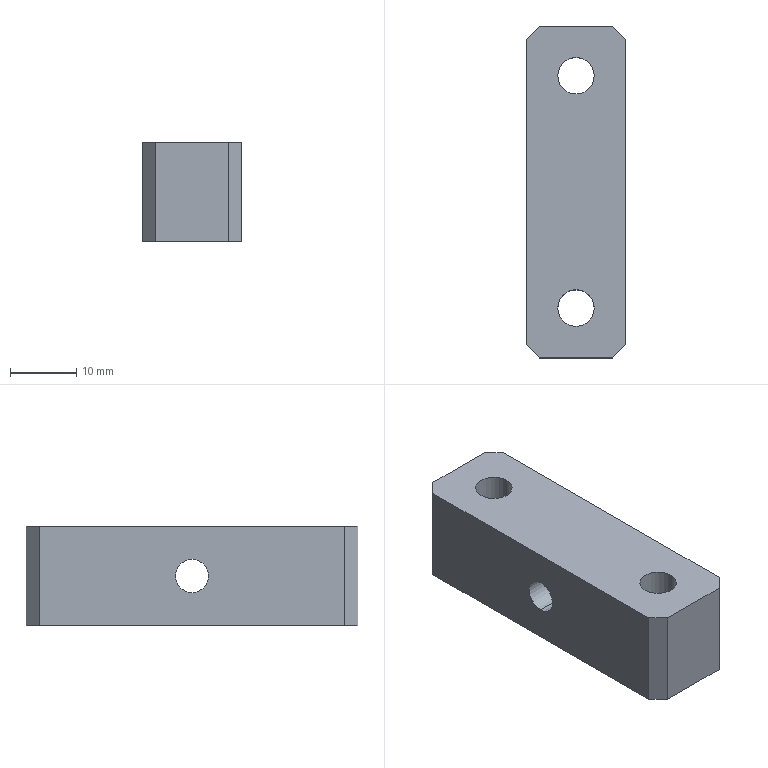Part | STEP file | MT-COMBO-119-S024 | 1 solid | 16 faces | box 15 x 50 x 15 mm | volume 10123 mm3 | plane 10 | cylinder 6 | commonest cylinder face diameters 5.5 x4 5 x2
STEP:
#1=CARTESIAN_POINT('',(0.,25.,5.));
#2=VERTEX_POINT('',#1);
#3=CARTESIAN_POINT('',(0.,25.,10.));
#4=VERTEX_POINT('',#3);
#5=CARTESIAN_POINT('',(0.,25.,7.5));
#6=DIRECTION('',(-1.,0.,0.));
#7=DIRECTION('',(0.,0.,1.));
#8=AXIS2_PLACEMENT_3D('',#5,#6,#7);
#9=CIRCLE('',#8,2.5);
#10=EDGE_CURVE('',#2,#4,#9,.T.);
#11=ORIENTED_EDGE('',*,*,#10,.F.);
#12=CARTESIAN_POINT('',(-15.,25.,5.));
#13=VERTEX_POINT('',#12);
#14=CARTESIAN_POINT('',(-15.,25.,5.));
#15=DIRECTION('',(-1.,0.,0.));
#16=VECTOR('',#15,1000.);
#17=LINE('',#14,#16);
#18=EDGE_CURVE('',#2,#13,#17,.T.);
#19=ORIENTED_EDGE('',*,*,#18,.T.);
#20=CARTESIAN_POINT('',(-15.,25.,10.));
#21=VERTEX_POINT('',#20);
#22=CARTESIAN_POINT('',(-15.,25.,7.5));
#23=DIRECTION('',(-1.,0.,0.));
#24=DIRECTION('',(0.,0.,1.));
#25=AXIS2_PLACEMENT_3D('',#22,#23,#24);
#26=CIRCLE('',#25,2.5);
#27=EDGE_CURVE('',#13,#21,#26,.T.);
#28=ORIENTED_EDGE('',*,*,#27,.T.);
#29=CARTESIAN_POINT('',(-15.,25.,10.));
#30=DIRECTION('',(-1.,0.,0.));
#31=VECTOR('',#30,1000.);
#32=LINE('',#29,#31);
#33=EDGE_CURVE('',#4,#21,#32,.T.);
#34=ORIENTED_EDGE('',*,*,#33,.F.);
#35=EDGE_LOOP('',(#11,#19,#28,#34));
#36=FACE_OUTER_BOUND('',#35,.T.);
#37=CARTESIAN_POINT('',(-15.,25.,7.5));
#38=DIRECTION('',(-1.,0.,0.));
#39=DIRECTION('',(0.,0.,1.));
#40=AXIS2_PLACEMENT_3D('',#37,#38,#39);
#41=CYLINDRICAL_SURFACE('',#40,2.5);
#42=ADVANCED_FACE('',(#36),#41,.F.);
#43=CARTESIAN_POINT('',(-10.25,7.5,0.));
#44=VERTEX_POINT('',#43);
#45=CARTESIAN_POINT('',(-4.75,7.5,0.));
#46=VERTEX_POINT('',#45);
#47=CARTESIAN_POINT('',(-7.5,7.5,0.));
#48=DIRECTION('',(0.,0.,1.));
#49=DIRECTION('',(1.,0.,0.));
#50=AXIS2_PLACEMENT_3D('',#47,#48,#49);
#51=CIRCLE('',#50,2.75);
#52=EDGE_CURVE('',#44,#46,#51,.T.);
#53=ORIENTED_EDGE('',*,*,#52,.F.);
#54=CARTESIAN_POINT('',(-10.25,7.5,15.));
#55=VERTEX_POINT('',#54);
#56=CARTESIAN_POINT('',(-10.25,7.5,15.));
#57=DIRECTION('',(0.,0.,1.));
#58=VECTOR('',#57,1000.);
#59=LINE('',#56,#58);
#60=EDGE_CURVE('',#44,#55,#59,.T.);
#61=ORIENTED_EDGE('',*,*,#60,.T.);
#62=CARTESIAN_POINT('',(-4.75,7.5,15.));
#63=VERTEX_POINT('',#62);
#64=CARTESIAN_POINT('',(-7.5,7.5,15.));
#65=DIRECTION('',(0.,0.,1.));
#66=DIRECTION('',(1.,0.,0.));
#67=AXIS2_PLACEMENT_3D('',#64,#65,#66);
#68=CIRCLE('',#67,2.75);
#69=EDGE_CURVE('',#55,#63,#68,.T.);
#70=ORIENTED_EDGE('',*,*,#69,.T.);
#71=CARTESIAN_POINT('',(-4.75,7.5,15.));
#72=DIRECTION('',(0.,0.,1.));
#73=VECTOR('',#72,1000.);
#74=LINE('',#71,#73);
#75=EDGE_CURVE('',#46,#63,#74,.T.);
#76=ORIENTED_EDGE('',*,*,#75,.F.);
#77=EDGE_LOOP('',(#53,#61,#70,#76));
#78=FACE_OUTER_BOUND('',#77,.T.);
#79=CARTESIAN_POINT('',(-7.5,7.5,15.));
#80=DIRECTION('',(0.,0.,1.));
#81=DIRECTION('',(1.,0.,0.));
#82=AXIS2_PLACEMENT_3D('',#79,#80,#81);
#83=CYLINDRICAL_SURFACE('',#82,2.75);
#84=ADVANCED_FACE('',(#78),#83,.F.);
#85=CARTESIAN_POINT('',(-10.25,42.5,0.));
#86=VERTEX_POINT('',#85);
#87=CARTESIAN_POINT('',(-4.75,42.5,0.));
#88=VERTEX_POINT('',#87);
#89=CARTESIAN_POINT('',(-7.5,42.5,0.));
#90=DIRECTION('',(0.,0.,1.));
#91=DIRECTION('',(1.,0.,0.));
#92=AXIS2_PLACEMENT_3D('',#89,#90,#91);
#93=CIRCLE('',#92,2.75);
#94=EDGE_CURVE('',#86,#88,#93,.T.);
#95=ORIENTED_EDGE('',*,*,#94,.F.);
#96=CARTESIAN_POINT('',(-10.25,42.5,15.));
#97=VERTEX_POINT('',#96);
#98=CARTESIAN_POINT('',(-10.25,42.5,15.));
#99=DIRECTION('',(0.,0.,1.));
#100=VECTOR('',#99,1000.);
#101=LINE('',#98,#100);
#102=EDGE_CURVE('',#86,#97,#101,.T.);
#103=ORIENTED_EDGE('',*,*,#102,.T.);
#104=CARTESIAN_POINT('',(-4.75,42.5,15.));
#105=VERTEX_POINT('',#104);
#106=CARTESIAN_POINT('',(-7.5,42.5,15.));
#107=DIRECTION('',(0.,0.,1.));
#108=DIRECTION('',(1.,0.,0.));
#109=AXIS2_PLACEMENT_3D('',#106,#107,#108);
#110=CIRCLE('',#109,2.75);
#111=EDGE_CURVE('',#97,#105,#110,.T.);
#112=ORIENTED_EDGE('',*,*,#111,.T.);
#113=CARTESIAN_POINT('',(-4.75,42.5,15.));
#114=DIRECTION('',(0.,0.,1.));
#115=VECTOR('',#114,1000.);
#116=LINE('',#113,#115);
#117=EDGE_CURVE('',#88,#105,#116,.T.);
#118=ORIENTED_EDGE('',*,*,#117,.F.);
#119=EDGE_LOOP('',(#95,#103,#112,#118));
#120=FACE_OUTER_BOUND('',#119,.T.);
#121=CARTESIAN_POINT('',(-7.5,42.5,15.));
#122=DIRECTION('',(0.,0.,1.));
#123=DIRECTION('',(1.,0.,0.));
#124=AXIS2_PLACEMENT_3D('',#121,#122,#123);
#125=CYLINDRICAL_SURFACE('',#124,2.75);
#126=ADVANCED_FACE('',(#120),#125,.F.);
#127=CARTESIAN_POINT('',(-15.,25.,7.5));
#128=DIRECTION('',(-1.,0.,0.));
#129=DIRECTION('',(0.,0.,1.));
#130=AXIS2_PLACEMENT_3D('',#127,#128,#129);
#131=CIRCLE('',#130,2.5);
#132=EDGE_CURVE('',#21,#13,#131,.T.);
#133=ORIENTED_EDGE('',*,*,#132,.F.);
#134=ORIENTED_EDGE('',*,*,#27,.F.);
#135=EDGE_LOOP('',(#133,#134));
#136=FACE_BOUND('',#135,.T.);
#137=CARTESIAN_POINT('',(-15.,48.,15.));
#138=VERTEX_POINT('',#137);
#139=CARTESIAN_POINT('',(-15.,2.,15.));
#140=VERTEX_POINT('',#139);
#141=CARTESIAN_POINT('',(-15.,50.,15.));
#142=DIRECTION('',(0.,-1.,0.));
#143=VECTOR('',#142,1000.);
#144=LINE('',#141,#143);
#145=EDGE_CURVE('',#138,#140,#144,.T.);
#146=ORIENTED_EDGE('',*,*,#145,.F.);
#147=CARTESIAN_POINT('',(-15.,48.,0.));
#148=VERTEX_POINT('',#147);
#149=CARTESIAN_POINT('',(-15.,48.,15.));
#150=DIRECTION('',(0.,0.,-1.));
#151=VECTOR('',#150,1000.);
#152=LINE('',#149,#151);
#153=EDGE_CURVE('',#138,#148,#152,.T.);
#154=ORIENTED_EDGE('',*,*,#153,.T.);
#155=CARTESIAN_POINT('',(-15.,2.,0.));
#156=VERTEX_POINT('',#155);
#157=CARTESIAN_POINT('',(-15.,50.,0.));
#158=DIRECTION('',(0.,-1.,0.));
#159=VECTOR('',#158,1000.);
#160=LINE('',#157,#159);
#161=EDGE_CURVE('',#148,#156,#160,.T.);
#162=ORIENTED_EDGE('',*,*,#161,.T.);
#163=CARTESIAN_POINT('',(-15.,2.,15.));
#164=DIRECTION('',(0.,0.,1.));
#165=VECTOR('',#164,1000.);
#166=LINE('',#163,#165);
#167=EDGE_CURVE('',#156,#140,#166,.T.);
#168=ORIENTED_EDGE('',*,*,#167,.T.);
#169=EDGE_LOOP('',(#146,#154,#162,#168));
#170=FACE_OUTER_BOUND('',#169,.T.);
#171=CARTESIAN_POINT('',(-15.,50.,15.));
#172=DIRECTION('',(1.,0.,0.));
#173=DIRECTION('',(0.,1.,0.));
#174=AXIS2_PLACEMENT_3D('',#171,#172,#173);
#175=PLANE('',#174);
#176=ADVANCED_FACE('',(#136,#170),#175,.F.);
#177=CARTESIAN_POINT('',(-13.,0.,15.));
#178=VERTEX_POINT('',#177);
#179=CARTESIAN_POINT('',(-2.,0.,15.));
#180=VERTEX_POINT('',#179);
#181=CARTESIAN_POINT('',(-15.,0.,15.));
#182=DIRECTION('',(1.,0.,0.));
#183=VECTOR('',#182,1000.);
#184=LINE('',#181,#183);
#185=EDGE_CURVE('',#178,#180,#184,.T.);
#186=ORIENTED_EDGE('',*,*,#185,.F.);
#187=CARTESIAN_POINT('',(-13.,0.,0.));
#188=VERTEX_POINT('',#187);
#189=CARTESIAN_POINT('',(-13.,0.,15.));
#190=DIRECTION('',(0.,0.,-1.));
#191=VECTOR('',#190,1000.);
#192=LINE('',#189,#191);
#193=EDGE_CURVE('',#178,#188,#192,.T.);
#194=ORIENTED_EDGE('',*,*,#193,.T.);
#195=CARTESIAN_POINT('',(-2.,0.,0.));
#196=VERTEX_POINT('',#195);
#197=CARTESIAN_POINT('',(-15.,0.,0.));
#198=DIRECTION('',(1.,0.,0.));
#199=VECTOR('',#198,1000.);
#200=LINE('',#197,#199);
#201=EDGE_CURVE('',#188,#196,#200,.T.);
#202=ORIENTED_EDGE('',*,*,#201,.T.);
#203=CARTESIAN_POINT('',(-2.,0.,15.));
#204=DIRECTION('',(0.,0.,1.));
#205=VECTOR('',#204,1000.);
#206=LINE('',#203,#205);
#207=EDGE_CURVE('',#196,#180,#206,.T.);
#208=ORIENTED_EDGE('',*,*,#207,.T.);
#209=EDGE_LOOP('',(#186,#194,#202,#208));
#210=FACE_OUTER_BOUND('',#209,.T.);
#211=CARTESIAN_POINT('',(-15.,0.,15.));
#212=DIRECTION('',(0.,1.,0.));
#213=DIRECTION('',(0.,0.,1.));
#214=AXIS2_PLACEMENT_3D('',#211,#212,#213);
#215=PLANE('',#214);
#216=ADVANCED_FACE('',(#210),#215,.F.);
#217=CARTESIAN_POINT('',(0.,25.,7.5));
#218=DIRECTION('',(-1.,0.,0.));
#219=DIRECTION('',(0.,0.,1.));
#220=AXIS2_PLACEMENT_3D('',#217,#218,#219);
#221=CIRCLE('',#220,2.5);
#222=EDGE_CURVE('',#4,#2,#221,.T.);
#223=ORIENTED_EDGE('',*,*,#222,.T.);
#224=ORIENTED_EDGE('',*,*,#10,.T.);
#225=EDGE_LOOP('',(#223,#224));
#226=FACE_BOUND('',#225,.T.);
#227=CARTESIAN_POINT('',(0.,2.,0.));
#228=VERTEX_POINT('',#227);
#229=CARTESIAN_POINT('',(0.,48.,0.));
#230=VERTEX_POINT('',#229);
#231=CARTESIAN_POINT('',(0.,50.,0.));
#232=DIRECTION('',(0.,1.,0.));
#233=VECTOR('',#232,1000.);
#234=LINE('',#231,#233);
#235=EDGE_CURVE('',#228,#230,#234,.T.);
#236=ORIENTED_EDGE('',*,*,#235,.T.);
#237=CARTESIAN_POINT('',(0.,48.,15.));
#238=VERTEX_POINT('',#237);
#239=CARTESIAN_POINT('',(0.,48.,15.));
#240=DIRECTION('',(0.,0.,1.));
#241=VECTOR('',#240,1000.);
#242=LINE('',#239,#241);
#243=EDGE_CURVE('',#230,#238,#242,.T.);
#244=ORIENTED_EDGE('',*,*,#243,.T.);
#245=CARTESIAN_POINT('',(0.,2.,15.));
#246=VERTEX_POINT('',#245);
#247=CARTESIAN_POINT('',(0.,50.,15.));
#248=DIRECTION('',(0.,1.,0.));
#249=VECTOR('',#248,1000.);
#250=LINE('',#247,#249);
#251=EDGE_CURVE('',#246,#238,#250,.T.);
#252=ORIENTED_EDGE('',*,*,#251,.F.);
#253=CARTESIAN_POINT('',(0.,2.,15.));
#254=DIRECTION('',(0.,0.,-1.));
#255=VECTOR('',#254,1000.);
#256=LINE('',#253,#255);
#257=EDGE_CURVE('',#246,#228,#256,.T.);
#258=ORIENTED_EDGE('',*,*,#257,.T.);
#259=EDGE_LOOP('',(#236,#244,#252,#258));
#260=FACE_OUTER_BOUND('',#259,.T.);
#261=CARTESIAN_POINT('',(0.,50.,15.));
#262=DIRECTION('',(-1.,0.,0.));
#263=DIRECTION('',(0.,-1.,0.));
#264=AXIS2_PLACEMENT_3D('',#261,#262,#263);
#265=PLANE('',#264);
#266=ADVANCED_FACE('',(#226,#260),#265,.F.);
#267=CARTESIAN_POINT('',(-2.,50.,15.));
#268=VERTEX_POINT('',#267);
#269=CARTESIAN_POINT('',(-13.,50.,15.));
#270=VERTEX_POINT('',#269);
#271=CARTESIAN_POINT('',(-15.,50.,15.));
#272=DIRECTION('',(-1.,0.,0.));
#273=VECTOR('',#272,1000.);
#274=LINE('',#271,#273);
#275=EDGE_CURVE('',#268,#270,#274,.T.);
#276=ORIENTED_EDGE('',*,*,#275,.F.);
#277=CARTESIAN_POINT('',(-2.,50.,0.));
#278=VERTEX_POINT('',#277);
#279=CARTESIAN_POINT('',(-2.,50.,15.));
#280=DIRECTION('',(0.,0.,-1.));
#281=VECTOR('',#280,1000.);
#282=LINE('',#279,#281);
#283=EDGE_CURVE('',#268,#278,#282,.T.);
#284=ORIENTED_EDGE('',*,*,#283,.T.);
#285=CARTESIAN_POINT('',(-13.,50.,0.));
#286=VERTEX_POINT('',#285);
#287=CARTESIAN_POINT('',(-15.,50.,0.));
#288=DIRECTION('',(-1.,0.,0.));
#289=VECTOR('',#288,1000.);
#290=LINE('',#287,#289);
#291=EDGE_CURVE('',#278,#286,#290,.T.);
#292=ORIENTED_EDGE('',*,*,#291,.T.);
#293=CARTESIAN_POINT('',(-13.,50.,15.));
#294=DIRECTION('',(0.,0.,1.));
#295=VECTOR('',#294,1000.);
#296=LINE('',#293,#295);
#297=EDGE_CURVE('',#286,#270,#296,.T.);
#298=ORIENTED_EDGE('',*,*,#297,.T.);
#299=EDGE_LOOP('',(#276,#284,#292,#298));
#300=FACE_OUTER_BOUND('',#299,.T.);
#301=CARTESIAN_POINT('',(-15.,50.,15.));
#302=DIRECTION('',(0.,-1.,0.));
#303=DIRECTION('',(0.,0.,-1.));
#304=AXIS2_PLACEMENT_3D('',#301,#302,#303);
#305=PLANE('',#304);
#306=ADVANCED_FACE('',(#300),#305,.F.);
#307=CARTESIAN_POINT('',(-7.5,7.5,15.));
#308=DIRECTION('',(0.,0.,1.));
#309=DIRECTION('',(1.,0.,0.));
#310=AXIS2_PLACEMENT_3D('',#307,#308,#309);
#311=CIRCLE('',#310,2.75);
#312=EDGE_CURVE('',#63,#55,#311,.T.);
#313=ORIENTED_EDGE('',*,*,#312,.F.);
#314=ORIENTED_EDGE('',*,*,#69,.F.);
#315=EDGE_LOOP('',(#313,#314));
#316=FACE_BOUND('',#315,.T.);
#317=CARTESIAN_POINT('',(-7.5,42.5,15.));
#318=DIRECTION('',(0.,0.,1.));
#319=DIRECTION('',(1.,0.,0.));
#320=AXIS2_PLACEMENT_3D('',#317,#318,#319);
#321=CIRCLE('',#320,2.75);
#322=EDGE_CURVE('',#105,#97,#321,.T.);
#323=ORIENTED_EDGE('',*,*,#322,.F.);
#324=ORIENTED_EDGE('',*,*,#111,.F.);
#325=EDGE_LOOP('',(#323,#324));
#326=FACE_BOUND('',#325,.T.);
#327=ORIENTED_EDGE('',*,*,#251,.T.);
#328=CARTESIAN_POINT('',(24.,24.,15.));
#329=DIRECTION('',(-0.7071,0.7071,0.));
#330=VECTOR('',#329,1000.);
#331=LINE('',#328,#330);
#332=EDGE_CURVE('',#238,#268,#331,.T.);
#333=ORIENTED_EDGE('',*,*,#332,.T.);
#334=ORIENTED_EDGE('',*,*,#275,.T.);
#335=CARTESIAN_POINT('',(-31.5,31.5,15.));
#336=DIRECTION('',(-0.7071,-0.7071,0.));
#337=VECTOR('',#336,1000.);
#338=LINE('',#335,#337);
#339=EDGE_CURVE('',#270,#138,#338,.T.);
#340=ORIENTED_EDGE('',*,*,#339,.T.);
#341=ORIENTED_EDGE('',*,*,#145,.T.);
#342=CARTESIAN_POINT('',(-6.5,-6.5,15.));
#343=DIRECTION('',(0.7071,-0.7071,0.));
#344=VECTOR('',#343,1000.);
#345=LINE('',#342,#344);
#346=EDGE_CURVE('',#140,#178,#345,.T.);
#347=ORIENTED_EDGE('',*,*,#346,.T.);
#348=ORIENTED_EDGE('',*,*,#185,.T.);
#349=CARTESIAN_POINT('',(-1.,1.,15.));
#350=DIRECTION('',(0.7071,0.7071,0.));
#351=VECTOR('',#350,1000.);
#352=LINE('',#349,#351);
#353=EDGE_CURVE('',#180,#246,#352,.T.);
#354=ORIENTED_EDGE('',*,*,#353,.T.);
#355=EDGE_LOOP('',(#327,#333,#334,#340,#341,#347,#348,#354));
#356=FACE_OUTER_BOUND('',#355,.T.);
#357=CARTESIAN_POINT('',(0.,0.,15.));
#358=DIRECTION('',(0.,0.,1.));
#359=DIRECTION('',(1.,0.,0.));
#360=AXIS2_PLACEMENT_3D('',#357,#358,#359);
#361=PLANE('',#360);
#362=ADVANCED_FACE('',(#316,#326,#356),#361,.T.);
#363=CARTESIAN_POINT('',(-7.5,7.5,0.));
#364=DIRECTION('',(0.,0.,1.));
#365=DIRECTION('',(1.,0.,0.));
#366=AXIS2_PLACEMENT_3D('',#363,#364,#365);
#367=CIRCLE('',#366,2.75);
#368=EDGE_CURVE('',#46,#44,#367,.T.);
#369=ORIENTED_EDGE('',*,*,#368,.T.);
#370=ORIENTED_EDGE('',*,*,#52,.T.);
#371=EDGE_LOOP('',(#369,#370));
#372=FACE_BOUND('',#371,.T.);
#373=CARTESIAN_POINT('',(-7.5,42.5,0.));
#374=DIRECTION('',(0.,0.,1.));
#375=DIRECTION('',(1.,0.,0.));
#376=AXIS2_PLACEMENT_3D('',#373,#374,#375);
#377=CIRCLE('',#376,2.75);
#378=EDGE_CURVE('',#88,#86,#377,.T.);
#379=ORIENTED_EDGE('',*,*,#378,.T.);
#380=ORIENTED_EDGE('',*,*,#94,.T.);
#381=EDGE_LOOP('',(#379,#380));
#382=FACE_BOUND('',#381,.T.);
#383=ORIENTED_EDGE('',*,*,#291,.F.);
#384=CARTESIAN_POINT('',(-2.,50.,0.));
#385=DIRECTION('',(0.7071,-0.7071,0.));
#386=VECTOR('',#385,1000.);
#387=LINE('',#384,#386);
#388=EDGE_CURVE('',#278,#230,#387,.T.);
#389=ORIENTED_EDGE('',*,*,#388,.T.);
#390=ORIENTED_EDGE('',*,*,#235,.F.);
#391=CARTESIAN_POINT('',(0.,2.,0.));
#392=DIRECTION('',(-0.7071,-0.7071,0.));
#393=VECTOR('',#392,1000.);
#394=LINE('',#391,#393);
#395=EDGE_CURVE('',#228,#196,#394,.T.);
#396=ORIENTED_EDGE('',*,*,#395,.T.);
#397=ORIENTED_EDGE('',*,*,#201,.F.);
#398=CARTESIAN_POINT('',(-13.,0.,0.));
#399=DIRECTION('',(-0.7071,0.7071,0.));
#400=VECTOR('',#399,1000.);
#401=LINE('',#398,#400);
#402=EDGE_CURVE('',#188,#156,#401,.T.);
#403=ORIENTED_EDGE('',*,*,#402,.T.);
#404=ORIENTED_EDGE('',*,*,#161,.F.);
#405=CARTESIAN_POINT('',(-15.,48.,0.));
#406=DIRECTION('',(0.7071,0.7071,0.));
#407=VECTOR('',#406,1000.);
#408=LINE('',#405,#407);
#409=EDGE_CURVE('',#148,#286,#408,.T.);
#410=ORIENTED_EDGE('',*,*,#409,.T.);
#411=EDGE_LOOP('',(#383,#389,#390,#396,#397,#403,#404,#410));
#412=FACE_OUTER_BOUND('',#411,.T.);
#413=CARTESIAN_POINT('',(0.,0.,0.));
#414=DIRECTION('',(0.,0.,1.));
#415=DIRECTION('',(1.,0.,0.));
#416=AXIS2_PLACEMENT_3D('',#413,#414,#415);
#417=PLANE('',#416);
#418=ADVANCED_FACE('',(#372,#382,#412),#417,.F.);
#419=ORIENTED_EDGE('',*,*,#102,.F.);
#420=ORIENTED_EDGE('',*,*,#378,.F.);
#421=ORIENTED_EDGE('',*,*,#117,.T.);
#422=ORIENTED_EDGE('',*,*,#322,.T.);
#423=EDGE_LOOP('',(#419,#420,#421,#422));
#424=FACE_OUTER_BOUND('',#423,.T.);
#425=CARTESIAN_POINT('',(-7.5,42.5,15.));
#426=DIRECTION('',(0.,0.,1.));
#427=DIRECTION('',(1.,0.,0.));
#428=AXIS2_PLACEMENT_3D('',#425,#426,#427);
#429=CYLINDRICAL_SURFACE('',#428,2.75);
#430=ADVANCED_FACE('',(#424),#429,.F.);
#431=ORIENTED_EDGE('',*,*,#60,.F.);
#432=ORIENTED_EDGE('',*,*,#368,.F.);
#433=ORIENTED_EDGE('',*,*,#75,.T.);
#434=ORIENTED_EDGE('',*,*,#312,.T.);
#435=EDGE_LOOP('',(#431,#432,#433,#434));
#436=FACE_OUTER_BOUND('',#435,.T.);
#437=CARTESIAN_POINT('',(-7.5,7.5,15.));
#438=DIRECTION('',(0.,0.,1.));
#439=DIRECTION('',(1.,0.,0.));
#440=AXIS2_PLACEMENT_3D('',#437,#438,#439);
#441=CYLINDRICAL_SURFACE('',#440,2.75);
#442=ADVANCED_FACE('',(#436),#441,.F.);
#443=ORIENTED_EDGE('',*,*,#332,.F.);
#444=ORIENTED_EDGE('',*,*,#243,.F.);
#445=ORIENTED_EDGE('',*,*,#388,.F.);
#446=ORIENTED_EDGE('',*,*,#283,.F.);
#447=EDGE_LOOP('',(#443,#444,#445,#446));
#448=FACE_OUTER_BOUND('',#447,.T.);
#449=CARTESIAN_POINT('',(-2.,50.,15.));
#450=DIRECTION('',(-0.7071,-0.7071,0.));
#451=DIRECTION('',(0.,0.,-1.));
#452=AXIS2_PLACEMENT_3D('',#449,#450,#451);
#453=PLANE('',#452);
#454=ADVANCED_FACE('',(#448),#453,.F.);
#455=ORIENTED_EDGE('',*,*,#339,.F.);
#456=ORIENTED_EDGE('',*,*,#297,.F.);
#457=ORIENTED_EDGE('',*,*,#409,.F.);
#458=ORIENTED_EDGE('',*,*,#153,.F.);
#459=EDGE_LOOP('',(#455,#456,#457,#458));
#460=FACE_OUTER_BOUND('',#459,.T.);
#461=CARTESIAN_POINT('',(-15.,48.,15.));
#462=DIRECTION('',(0.7071,-0.7071,0.));
#463=DIRECTION('',(0.,0.,-1.));
#464=AXIS2_PLACEMENT_3D('',#461,#462,#463);
#465=PLANE('',#464);
#466=ADVANCED_FACE('',(#460),#465,.F.);
#467=ORIENTED_EDGE('',*,*,#346,.F.);
#468=ORIENTED_EDGE('',*,*,#167,.F.);
#469=ORIENTED_EDGE('',*,*,#402,.F.);
#470=ORIENTED_EDGE('',*,*,#193,.F.);
#471=EDGE_LOOP('',(#467,#468,#469,#470));
#472=FACE_OUTER_BOUND('',#471,.T.);
#473=CARTESIAN_POINT('',(-13.,0.,15.));
#474=DIRECTION('',(0.7071,0.7071,0.));
#475=DIRECTION('',(0.,0.,-1.));
#476=AXIS2_PLACEMENT_3D('',#473,#474,#475);
#477=PLANE('',#476);
#478=ADVANCED_FACE('',(#472),#477,.F.);
#479=ORIENTED_EDGE('',*,*,#353,.F.);
#480=ORIENTED_EDGE('',*,*,#207,.F.);
#481=ORIENTED_EDGE('',*,*,#395,.F.);
#482=ORIENTED_EDGE('',*,*,#257,.F.);
#483=EDGE_LOOP('',(#479,#480,#481,#482));
#484=FACE_OUTER_BOUND('',#483,.T.);
#485=CARTESIAN_POINT('',(0.,2.,15.));
#486=DIRECTION('',(-0.7071,0.7071,0.));
#487=DIRECTION('',(0.,0.,-1.));
#488=AXIS2_PLACEMENT_3D('',#485,#486,#487);
#489=PLANE('',#488);
#490=ADVANCED_FACE('',(#484),#489,.F.);
#491=ORIENTED_EDGE('',*,*,#18,.F.);
#492=ORIENTED_EDGE('',*,*,#222,.F.);
#493=ORIENTED_EDGE('',*,*,#33,.T.);
#494=ORIENTED_EDGE('',*,*,#132,.T.);
#495=EDGE_LOOP('',(#491,#492,#493,#494));
#496=FACE_OUTER_BOUND('',#495,.T.);
#497=CARTESIAN_POINT('',(-15.,25.,7.5));
#498=DIRECTION('',(-1.,0.,0.));
#499=DIRECTION('',(0.,0.,1.));
#500=AXIS2_PLACEMENT_3D('',#497,#498,#499);
#501=CYLINDRICAL_SURFACE('',#500,2.5);
#502=ADVANCED_FACE('',(#496),#501,.F.);
#503=CLOSED_SHELL('',(#42,#84,#126,#176,#216,#266,#306,#362,#418,#430,#442,#454,#466,#478,#490,#502));
#504=MANIFOLD_SOLID_BREP('',#503);
#505=CARTESIAN_POINT('',(0.,0.,0.));
#506=DIRECTION('',(0.,0.,1.));
#507=DIRECTION('',(1.,0.,0.));
#508=AXIS2_PLACEMENT_3D('',#505,#506,#507);
#509=(LENGTH_UNIT()NAMED_UNIT(*)SI_UNIT(.MILLI.,.METRE.));
#510=UNCERTAINTY_MEASURE_WITH_UNIT(LENGTH_MEASURE(0.00001),#509,'','');
#511=(NAMED_UNIT(*)PLANE_ANGLE_UNIT()SI_UNIT($,.RADIAN.));
#512=(NAMED_UNIT(*)SI_UNIT($,.STERADIAN.)SOLID_ANGLE_UNIT());
#513=(GEOMETRIC_REPRESENTATION_CONTEXT(3)GLOBAL_UNCERTAINTY_ASSIGNED_CONTEXT((#510))GLOBAL_UNIT_ASSIGNED_CONTEXT((#509,#511,#512))REPRESENTATION_CONTEXT('',''));
#514=ADVANCED_BREP_SHAPE_REPRESENTATION('',(#504,#508),#513);